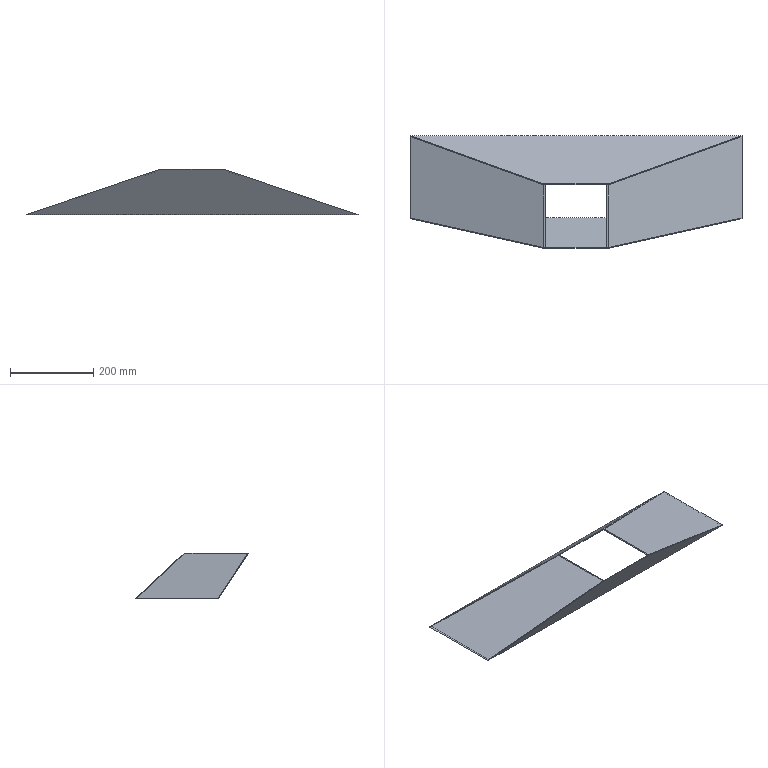Part | SolidWorks | features BaseBody 4 | 4 solids | 26 faces | box 800 x 271.5 x 109 mm | volume 384675 mm3 | plane 26
STEP:
#1=CARTESIAN_POINT('',(-400.,-98.206,0.));
#2=VERTEX_POINT('',#1);
#3=CARTESIAN_POINT('',(400.,-98.206,0.));
#4=VERTEX_POINT('',#3);
#5=CARTESIAN_POINT('',(0.,-98.206,0.));
#6=DIRECTION('',(1.,0.,0.));
#7=VECTOR('',#6,1000.);
#8=LINE('',#5,#7);
#9=EDGE_CURVE('',#2,#4,#8,.T.);
#10=ORIENTED_EDGE('',*,*,#9,.F.);
#11=CARTESIAN_POINT('',(-77.5,-169.706,109.));
#12=VERTEX_POINT('',#11);
#13=CARTESIAN_POINT('',(-74.891,-170.284,109.882));
#14=DIRECTION('',(-0.9271,0.2055,-0.3134));
#15=VECTOR('',#14,1000.);
#16=LINE('',#13,#15);
#17=EDGE_CURVE('',#12,#2,#16,.T.);
#18=ORIENTED_EDGE('',*,*,#17,.F.);
#19=CARTESIAN_POINT('',(77.5,-169.706,109.));
#20=VERTEX_POINT('',#19);
#21=CARTESIAN_POINT('',(0.,-169.706,109.));
#22=DIRECTION('',(1.,0.,0.));
#23=VECTOR('',#22,1000.);
#24=LINE('',#21,#23);
#25=EDGE_CURVE('',#12,#20,#24,.T.);
#26=ORIENTED_EDGE('',*,*,#25,.T.);
#27=CARTESIAN_POINT('',(74.891,-170.284,109.882));
#28=DIRECTION('',(-0.9271,-0.2055,0.3134));
#29=VECTOR('',#28,1000.);
#30=LINE('',#27,#29);
#31=EDGE_CURVE('',#4,#20,#30,.T.);
#32=ORIENTED_EDGE('',*,*,#31,.F.);
#33=EDGE_LOOP('',(#10,#18,#26,#32));
#34=FACE_OUTER_BOUND('',#33,.T.);
#35=CARTESIAN_POINT('',(-72.815,-169.706,109.));
#36=DIRECTION('',(0.,0.8362,0.5485));
#37=DIRECTION('',(1.,0.,0.));
#38=AXIS2_PLACEMENT_3D('',#35,#36,#37);
#39=PLANE('',#38);
#40=ADVANCED_FACE('',(#34),#39,.T.);
#41=ORIENTED_EDGE('',*,*,#25,.F.);
#42=CARTESIAN_POINT('',(-77.5,-171.5,109.));
#43=VERTEX_POINT('',#42);
#44=CARTESIAN_POINT('',(-77.5,-169.706,109.));
#45=CARTESIAN_POINT('',(-77.5,-170.304,109.));
#46=CARTESIAN_POINT('',(-77.5,-170.902,109.));
#47=CARTESIAN_POINT('',(-77.5,-171.5,109.));
#48=B_SPLINE_CURVE_WITH_KNOTS('',3,(#44,#45,#46,#47),.UNSPECIFIED.,.F.,.F.,(4,4),(0.9884,1.),.UNSPECIFIED.);
#49=EDGE_CURVE('',#12,#43,#48,.T.);
#50=ORIENTED_EDGE('',*,*,#49,.T.);
#51=CARTESIAN_POINT('',(77.5,-171.5,109.));
#52=VERTEX_POINT('',#51);
#53=CARTESIAN_POINT('',(-77.5,-171.5,109.));
#54=CARTESIAN_POINT('',(-25.833,-171.5,109.));
#55=CARTESIAN_POINT('',(25.833,-171.5,109.));
#56=CARTESIAN_POINT('',(77.5,-171.5,109.));
#57=B_SPLINE_CURVE_WITH_KNOTS('',3,(#53,#54,#55,#56),.UNSPECIFIED.,.F.,.F.,(4,4),(0.,1.),.UNSPECIFIED.);
#58=EDGE_CURVE('',#43,#52,#57,.T.);
#59=ORIENTED_EDGE('',*,*,#58,.T.);
#60=CARTESIAN_POINT('',(77.5,-171.5,109.));
#61=CARTESIAN_POINT('',(77.5,-170.902,109.));
#62=CARTESIAN_POINT('',(77.5,-170.304,109.));
#63=CARTESIAN_POINT('',(77.5,-169.706,109.));
#64=B_SPLINE_CURVE_WITH_KNOTS('',3,(#60,#61,#62,#63),.UNSPECIFIED.,.F.,.F.,(4,4),(0.,0.01157),.UNSPECIFIED.);
#65=EDGE_CURVE('',#52,#20,#64,.T.);
#66=ORIENTED_EDGE('',*,*,#65,.T.);
#67=EDGE_LOOP('',(#41,#50,#59,#66));
#68=FACE_OUTER_BOUND('',#67,.T.);
#69=CARTESIAN_POINT('',(0.,0.,109.));
#70=DIRECTION('',(0.,0.,-1.));
#71=DIRECTION('',(0.,-1.,0.));
#72=AXIS2_PLACEMENT_3D('',#69,#70,#71);
#73=PLANE('',#72);
#74=ADVANCED_FACE('',(#68),#73,.F.);
#75=CARTESIAN_POINT('',(-400.,-100.,0.));
#76=VERTEX_POINT('',#75);
#77=CARTESIAN_POINT('',(-400.,-98.206,0.));
#78=CARTESIAN_POINT('',(-400.,-98.804,0.));
#79=CARTESIAN_POINT('',(-400.,-99.402,0.));
#80=CARTESIAN_POINT('',(-400.,-100.,0.));
#81=B_SPLINE_CURVE_WITH_KNOTS('',3,(#77,#78,#79,#80),.UNSPECIFIED.,.F.,.F.,(4,4),(0.991,1.),.UNSPECIFIED.);
#82=EDGE_CURVE('',#2,#76,#81,.T.);
#83=ORIENTED_EDGE('',*,*,#82,.F.);
#84=ORIENTED_EDGE('',*,*,#9,.T.);
#85=CARTESIAN_POINT('',(400.,-100.,0.));
#86=VERTEX_POINT('',#85);
#87=CARTESIAN_POINT('',(400.,-100.,0.));
#88=CARTESIAN_POINT('',(400.,-99.402,0.));
#89=CARTESIAN_POINT('',(400.,-98.804,0.));
#90=CARTESIAN_POINT('',(400.,-98.206,0.));
#91=B_SPLINE_CURVE_WITH_KNOTS('',3,(#87,#88,#89,#90),.UNSPECIFIED.,.F.,.F.,(4,4),(0.,0.00897),.UNSPECIFIED.);
#92=EDGE_CURVE('',#86,#4,#91,.T.);
#93=ORIENTED_EDGE('',*,*,#92,.F.);
#94=CARTESIAN_POINT('',(-400.,-100.,0.));
#95=CARTESIAN_POINT('',(-133.333,-100.,0.));
#96=CARTESIAN_POINT('',(133.333,-100.,0.));
#97=CARTESIAN_POINT('',(400.,-100.,0.));
#98=B_SPLINE_CURVE_WITH_KNOTS('',3,(#94,#95,#96,#97),.UNSPECIFIED.,.F.,.F.,(4,4),(0.,1.),.UNSPECIFIED.);
#99=EDGE_CURVE('',#76,#86,#98,.T.);
#100=ORIENTED_EDGE('',*,*,#99,.F.);
#101=EDGE_LOOP('',(#83,#84,#93,#100));
#102=FACE_OUTER_BOUND('',#101,.T.);
#103=CARTESIAN_POINT('',(0.,0.,0.));
#104=DIRECTION('',(0.,0.,-1.));
#105=DIRECTION('',(0.,-1.,0.));
#106=AXIS2_PLACEMENT_3D('',#103,#104,#105);
#107=PLANE('',#106);
#108=ADVANCED_FACE('',(#102),#107,.T.);
#109=ORIENTED_EDGE('',*,*,#49,.F.);
#110=ORIENTED_EDGE('',*,*,#17,.T.);
#111=ORIENTED_EDGE('',*,*,#82,.T.);
#112=CARTESIAN_POINT('',(-77.5,-171.5,109.));
#113=DIRECTION('',(-0.9271,0.2055,-0.3134));
#114=VECTOR('',#113,1000.);
#115=LINE('',#112,#114);
#116=EDGE_CURVE('',#43,#76,#115,.T.);
#117=ORIENTED_EDGE('',*,*,#116,.F.);
#118=EDGE_LOOP('',(#109,#110,#111,#117));
#119=FACE_OUTER_BOUND('',#118,.T.);
#120=CARTESIAN_POINT('',(-41.009,0.,121.333));
#121=DIRECTION('',(-0.3202,0.,0.9474));
#122=DIRECTION('',(0.,1.,0.));
#123=AXIS2_PLACEMENT_3D('',#120,#121,#122);
#124=PLANE('',#123);
#125=ADVANCED_FACE('',(#119),#124,.T.);
#126=ORIENTED_EDGE('',*,*,#92,.T.);
#127=ORIENTED_EDGE('',*,*,#31,.T.);
#128=ORIENTED_EDGE('',*,*,#65,.F.);
#129=CARTESIAN_POINT('',(77.5,-171.5,109.));
#130=DIRECTION('',(0.9271,0.2055,-0.3134));
#131=VECTOR('',#130,1000.);
#132=LINE('',#129,#131);
#133=EDGE_CURVE('',#52,#86,#132,.T.);
#134=ORIENTED_EDGE('',*,*,#133,.T.);
#135=EDGE_LOOP('',(#126,#127,#128,#134));
#136=FACE_OUTER_BOUND('',#135,.T.);
#137=CARTESIAN_POINT('',(41.009,0.,121.333));
#138=DIRECTION('',(0.3202,0.,0.9474));
#139=DIRECTION('',(0.,-1.,0.));
#140=AXIS2_PLACEMENT_3D('',#137,#138,#139);
#141=PLANE('',#140);
#142=ADVANCED_FACE('',(#136),#141,.T.);
#143=ORIENTED_EDGE('',*,*,#116,.T.);
#144=ORIENTED_EDGE('',*,*,#99,.T.);
#145=ORIENTED_EDGE('',*,*,#133,.F.);
#146=ORIENTED_EDGE('',*,*,#58,.F.);
#147=EDGE_LOOP('',(#143,#144,#145,#146));
#148=FACE_OUTER_BOUND('',#147,.T.);
#149=CARTESIAN_POINT('',(0.,-69.916,-45.862));
#150=DIRECTION('',(0.,-0.8362,-0.5485));
#151=DIRECTION('',(0.,0.5485,-0.8362));
#152=AXIS2_PLACEMENT_3D('',#149,#150,#151);
#153=PLANE('',#152);
#154=ADVANCED_FACE('',(#148),#153,.T.);
#155=CLOSED_SHELL('',(#40,#74,#108,#125,#142,#154));
#156=MANIFOLD_SOLID_BREP('',#155);
#157=CARTESIAN_POINT('',(-400.,97.804,0.));
#158=VERTEX_POINT('',#157);
#159=CARTESIAN_POINT('',(-77.5,-18.696,109.));
#160=VERTEX_POINT('',#159);
#161=CARTESIAN_POINT('',(-50.26,-28.536,118.207));
#162=DIRECTION('',(0.8963,-0.3238,0.3029));
#163=VECTOR('',#162,1000.);
#164=LINE('',#161,#163);
#165=EDGE_CURVE('',#158,#160,#164,.T.);
#166=ORIENTED_EDGE('',*,*,#165,.F.);
#167=CARTESIAN_POINT('',(400.,97.804,0.));
#168=VERTEX_POINT('',#167);
#169=CARTESIAN_POINT('',(0.,97.804,0.));
#170=DIRECTION('',(-1.,0.,0.));
#171=VECTOR('',#170,1000.);
#172=LINE('',#169,#171);
#173=EDGE_CURVE('',#168,#158,#172,.T.);
#174=ORIENTED_EDGE('',*,*,#173,.F.);
#175=CARTESIAN_POINT('',(77.5,-18.696,109.));
#176=VERTEX_POINT('',#175);
#177=CARTESIAN_POINT('',(50.26,-28.536,118.207));
#178=DIRECTION('',(0.8963,0.3238,-0.3029));
#179=VECTOR('',#178,1000.);
#180=LINE('',#177,#179);
#181=EDGE_CURVE('',#176,#168,#180,.T.);
#182=ORIENTED_EDGE('',*,*,#181,.F.);
#183=CARTESIAN_POINT('',(0.,-18.696,109.));
#184=DIRECTION('',(-1.,0.,0.));
#185=VECTOR('',#184,1000.);
#186=LINE('',#183,#185);
#187=EDGE_CURVE('',#176,#160,#186,.T.);
#188=ORIENTED_EDGE('',*,*,#187,.T.);
#189=EDGE_LOOP('',(#166,#174,#182,#188));
#190=FACE_OUTER_BOUND('',#189,.T.);
#191=CARTESIAN_POINT('',(72.815,-18.696,109.));
#192=DIRECTION('',(0.,-0.6832,-0.7302));
#193=DIRECTION('',(0.,-0.7302,0.6832));
#194=AXIS2_PLACEMENT_3D('',#191,#192,#193);
#195=PLANE('',#194);
#196=ADVANCED_FACE('',(#190),#195,.T.);
#197=CARTESIAN_POINT('',(77.5,-16.5,109.));
#198=VERTEX_POINT('',#197);
#199=CARTESIAN_POINT('',(400.,100.,0.));
#200=VERTEX_POINT('',#199);
#201=CARTESIAN_POINT('',(77.5,-16.5,109.));
#202=DIRECTION('',(0.8963,0.3238,-0.3029));
#203=VECTOR('',#202,1000.);
#204=LINE('',#201,#203);
#205=EDGE_CURVE('',#198,#200,#204,.T.);
#206=ORIENTED_EDGE('',*,*,#205,.T.);
#207=CARTESIAN_POINT('',(-400.,100.,0.));
#208=VERTEX_POINT('',#207);
#209=CARTESIAN_POINT('',(400.,100.,0.));
#210=CARTESIAN_POINT('',(133.333,100.,0.));
#211=CARTESIAN_POINT('',(-133.333,100.,0.));
#212=CARTESIAN_POINT('',(-400.,100.,0.));
#213=B_SPLINE_CURVE_WITH_KNOTS('',3,(#209,#210,#211,#212),.UNSPECIFIED.,.F.,.F.,(4,4),(0.,1.),.UNSPECIFIED.);
#214=EDGE_CURVE('',#200,#208,#213,.T.);
#215=ORIENTED_EDGE('',*,*,#214,.T.);
#216=CARTESIAN_POINT('',(-77.5,-16.5,109.));
#217=VERTEX_POINT('',#216);
#218=CARTESIAN_POINT('',(-77.5,-16.5,109.));
#219=DIRECTION('',(-0.8963,0.3238,-0.3029));
#220=VECTOR('',#219,1000.);
#221=LINE('',#218,#220);
#222=EDGE_CURVE('',#217,#208,#221,.T.);
#223=ORIENTED_EDGE('',*,*,#222,.F.);
#224=CARTESIAN_POINT('',(77.5,-16.5,109.));
#225=CARTESIAN_POINT('',(25.833,-16.5,109.));
#226=CARTESIAN_POINT('',(-25.833,-16.5,109.));
#227=CARTESIAN_POINT('',(-77.5,-16.5,109.));
#228=B_SPLINE_CURVE_WITH_KNOTS('',3,(#224,#225,#226,#227),.UNSPECIFIED.,.F.,.F.,(4,4),(0.,1.),.UNSPECIFIED.);
#229=EDGE_CURVE('',#198,#217,#228,.T.);
#230=ORIENTED_EDGE('',*,*,#229,.F.);
#231=EDGE_LOOP('',(#206,#215,#223,#230));
#232=FACE_OUTER_BOUND('',#231,.T.);
#233=CARTESIAN_POINT('',(0.,46.678,49.89));
#234=DIRECTION('',(0.,0.6832,0.7302));
#235=DIRECTION('',(1.,0.,0.));
#236=AXIS2_PLACEMENT_3D('',#233,#234,#235);
#237=PLANE('',#236);
#238=ADVANCED_FACE('',(#232),#237,.T.);
#239=CARTESIAN_POINT('',(77.5,-18.696,109.));
#240=CARTESIAN_POINT('',(77.5,-17.964,109.));
#241=CARTESIAN_POINT('',(77.5,-17.232,109.));
#242=CARTESIAN_POINT('',(77.5,-16.5,109.));
#243=B_SPLINE_CURVE_WITH_KNOTS('',3,(#239,#240,#241,#242),.UNSPECIFIED.,.F.,.F.,(4,4),(0.9858,1.),.UNSPECIFIED.);
#244=EDGE_CURVE('',#176,#198,#243,.T.);
#245=ORIENTED_EDGE('',*,*,#244,.F.);
#246=ORIENTED_EDGE('',*,*,#181,.T.);
#247=CARTESIAN_POINT('',(400.,97.804,0.));
#248=CARTESIAN_POINT('',(400.,98.536,0.));
#249=CARTESIAN_POINT('',(400.,99.268,0.));
#250=CARTESIAN_POINT('',(400.,100.,0.));
#251=B_SPLINE_CURVE_WITH_KNOTS('',3,(#247,#248,#249,#250),.UNSPECIFIED.,.F.,.F.,(4,4),(0.989,1.),.UNSPECIFIED.);
#252=EDGE_CURVE('',#168,#200,#251,.T.);
#253=ORIENTED_EDGE('',*,*,#252,.T.);
#254=ORIENTED_EDGE('',*,*,#205,.F.);
#255=EDGE_LOOP('',(#245,#246,#253,#254));
#256=FACE_OUTER_BOUND('',#255,.T.);
#257=CARTESIAN_POINT('',(41.009,0.,121.333));
#258=DIRECTION('',(0.3202,0.,0.9474));
#259=DIRECTION('',(0.,-1.,0.));
#260=AXIS2_PLACEMENT_3D('',#257,#258,#259);
#261=PLANE('',#260);
#262=ADVANCED_FACE('',(#256),#261,.T.);
#263=CARTESIAN_POINT('',(-400.,100.,0.));
#264=CARTESIAN_POINT('',(-400.,99.268,0.));
#265=CARTESIAN_POINT('',(-400.,98.536,0.));
#266=CARTESIAN_POINT('',(-400.,97.804,0.));
#267=B_SPLINE_CURVE_WITH_KNOTS('',3,(#263,#264,#265,#266),.UNSPECIFIED.,.F.,.F.,(4,4),(0.,0.01098),.UNSPECIFIED.);
#268=EDGE_CURVE('',#208,#158,#267,.T.);
#269=ORIENTED_EDGE('',*,*,#268,.T.);
#270=ORIENTED_EDGE('',*,*,#165,.T.);
#271=CARTESIAN_POINT('',(-77.5,-16.5,109.));
#272=CARTESIAN_POINT('',(-77.5,-17.232,109.));
#273=CARTESIAN_POINT('',(-77.5,-17.964,109.));
#274=CARTESIAN_POINT('',(-77.5,-18.696,109.));
#275=B_SPLINE_CURVE_WITH_KNOTS('',3,(#271,#272,#273,#274),.UNSPECIFIED.,.F.,.F.,(4,4),(0.,0.01416),.UNSPECIFIED.);
#276=EDGE_CURVE('',#217,#160,#275,.T.);
#277=ORIENTED_EDGE('',*,*,#276,.F.);
#278=ORIENTED_EDGE('',*,*,#222,.T.);
#279=EDGE_LOOP('',(#269,#270,#277,#278));
#280=FACE_OUTER_BOUND('',#279,.T.);
#281=CARTESIAN_POINT('',(-41.009,0.,121.333));
#282=DIRECTION('',(-0.3202,0.,0.9474));
#283=DIRECTION('',(0.,1.,0.));
#284=AXIS2_PLACEMENT_3D('',#281,#282,#283);
#285=PLANE('',#284);
#286=ADVANCED_FACE('',(#280),#285,.T.);
#287=ORIENTED_EDGE('',*,*,#187,.F.);
#288=ORIENTED_EDGE('',*,*,#244,.T.);
#289=ORIENTED_EDGE('',*,*,#229,.T.);
#290=ORIENTED_EDGE('',*,*,#276,.T.);
#291=EDGE_LOOP('',(#287,#288,#289,#290));
#292=FACE_OUTER_BOUND('',#291,.T.);
#293=CARTESIAN_POINT('',(0.,0.,109.));
#294=DIRECTION('',(0.,0.,-1.));
#295=DIRECTION('',(0.,-1.,0.));
#296=AXIS2_PLACEMENT_3D('',#293,#294,#295);
#297=PLANE('',#296);
#298=ADVANCED_FACE('',(#292),#297,.F.);
#299=ORIENTED_EDGE('',*,*,#252,.F.);
#300=ORIENTED_EDGE('',*,*,#173,.T.);
#301=ORIENTED_EDGE('',*,*,#268,.F.);
#302=ORIENTED_EDGE('',*,*,#214,.F.);
#303=EDGE_LOOP('',(#299,#300,#301,#302));
#304=FACE_OUTER_BOUND('',#303,.T.);
#305=CARTESIAN_POINT('',(0.,0.,0.));
#306=DIRECTION('',(0.,0.,-1.));
#307=DIRECTION('',(0.,-1.,0.));
#308=AXIS2_PLACEMENT_3D('',#305,#306,#307);
#309=PLANE('',#308);
#310=ADVANCED_FACE('',(#304),#309,.T.);
#311=CLOSED_SHELL('',(#196,#238,#262,#286,#298,#310));
#312=MANIFOLD_SOLID_BREP('',#311);
#313=CARTESIAN_POINT('',(74.615,-169.706,109.));
#314=VERTEX_POINT('',#313);
#315=CARTESIAN_POINT('',(74.615,-18.696,109.));
#316=VERTEX_POINT('',#315);
#317=CARTESIAN_POINT('',(74.615,0.,109.));
#318=DIRECTION('',(0.,1.,0.));
#319=VECTOR('',#318,1000.);
#320=LINE('',#317,#319);
#321=EDGE_CURVE('',#314,#316,#320,.T.);
#322=ORIENTED_EDGE('',*,*,#321,.T.);
#323=CARTESIAN_POINT('',(74.615,-18.045,108.392));
#324=VERTEX_POINT('',#323);
#325=CARTESIAN_POINT('',(74.615,-11.983,102.72));
#326=DIRECTION('',(0.,-0.7302,0.6832));
#327=VECTOR('',#326,1000.);
#328=LINE('',#325,#327);
#329=EDGE_CURVE('',#324,#316,#328,.T.);
#330=ORIENTED_EDGE('',*,*,#329,.F.);
#331=CARTESIAN_POINT('',(74.615,-169.307,108.392));
#332=VERTEX_POINT('',#331);
#333=CARTESIAN_POINT('',(74.615,0.,108.392));
#334=DIRECTION('',(0.,-1.,0.));
#335=VECTOR('',#334,1000.);
#336=LINE('',#333,#335);
#337=EDGE_CURVE('',#324,#332,#336,.T.);
#338=ORIENTED_EDGE('',*,*,#337,.T.);
#339=CARTESIAN_POINT('',(74.615,-165.587,102.72));
#340=DIRECTION('',(0.,0.5485,-0.8362));
#341=VECTOR('',#340,1000.);
#342=LINE('',#339,#341);
#343=EDGE_CURVE('',#314,#332,#342,.T.);
#344=ORIENTED_EDGE('',*,*,#343,.F.);
#345=EDGE_LOOP('',(#322,#330,#338,#344));
#346=FACE_OUTER_BOUND('',#345,.T.);
#347=CARTESIAN_POINT('',(74.615,0.,0.));
#348=DIRECTION('',(-1.,0.,0.));
#349=DIRECTION('',(0.,0.,1.));
#350=AXIS2_PLACEMENT_3D('',#347,#348,#349);
#351=PLANE('',#350);
#352=ADVANCED_FACE('',(#346),#351,.T.);
#353=CARTESIAN_POINT('',(400.,97.804,0.));
#354=VERTEX_POINT('',#353);
#355=CARTESIAN_POINT('',(395.315,97.804,0.));
#356=VERTEX_POINT('',#355);
#357=CARTESIAN_POINT('',(0.,97.804,0.));
#358=DIRECTION('',(-1.,0.,0.));
#359=VECTOR('',#358,1000.);
#360=LINE('',#357,#359);
#361=EDGE_CURVE('',#354,#356,#360,.T.);
#362=ORIENTED_EDGE('',*,*,#361,.F.);
#363=CARTESIAN_POINT('',(400.,-98.206,0.));
#364=VERTEX_POINT('',#363);
#365=CARTESIAN_POINT('',(400.,-98.206,0.));
#366=CARTESIAN_POINT('',(400.,-32.869,0.));
#367=CARTESIAN_POINT('',(400.,32.468,0.));
#368=CARTESIAN_POINT('',(400.,97.804,0.));
#369=B_SPLINE_CURVE_WITH_KNOTS('',3,(#365,#366,#367,#368),.UNSPECIFIED.,.F.,.F.,(4,4),(0.00897,0.989),.UNSPECIFIED.);
#370=EDGE_CURVE('',#364,#354,#369,.T.);
#371=ORIENTED_EDGE('',*,*,#370,.F.);
#372=CARTESIAN_POINT('',(395.315,-98.206,0.));
#373=VERTEX_POINT('',#372);
#374=CARTESIAN_POINT('',(0.,-98.206,0.));
#375=DIRECTION('',(1.,0.,0.));
#376=VECTOR('',#375,1000.);
#377=LINE('',#374,#376);
#378=EDGE_CURVE('',#373,#364,#377,.T.);
#379=ORIENTED_EDGE('',*,*,#378,.F.);
#380=CARTESIAN_POINT('',(395.315,0.,0.));
#381=DIRECTION('',(0.,1.,0.));
#382=VECTOR('',#381,1000.);
#383=LINE('',#380,#382);
#384=EDGE_CURVE('',#373,#356,#383,.T.);
#385=ORIENTED_EDGE('',*,*,#384,.T.);
#386=EDGE_LOOP('',(#362,#371,#379,#385));
#387=FACE_OUTER_BOUND('',#386,.T.);
#388=CARTESIAN_POINT('',(0.,0.,0.));
#389=DIRECTION('',(0.,0.,-1.));
#390=DIRECTION('',(0.,-1.,0.));
#391=AXIS2_PLACEMENT_3D('',#388,#389,#390);
#392=PLANE('',#391);
#393=ADVANCED_FACE('',(#387),#392,.T.);
#394=CARTESIAN_POINT('',(77.5,-18.696,109.));
#395=VERTEX_POINT('',#394);
#396=CARTESIAN_POINT('',(50.26,-28.536,118.207));
#397=DIRECTION('',(0.8963,0.3238,-0.3029));
#398=VECTOR('',#397,1000.);
#399=LINE('',#396,#398);
#400=EDGE_CURVE('',#395,#354,#399,.T.);
#401=ORIENTED_EDGE('',*,*,#400,.F.);
#402=CARTESIAN_POINT('',(77.5,-169.706,109.));
#403=VERTEX_POINT('',#402);
#404=CARTESIAN_POINT('',(77.5,-169.706,109.));
#405=CARTESIAN_POINT('',(77.5,-119.369,109.));
#406=CARTESIAN_POINT('',(77.5,-69.032,109.));
#407=CARTESIAN_POINT('',(77.5,-18.696,109.));
#408=B_SPLINE_CURVE_WITH_KNOTS('',3,(#404,#405,#406,#407),.UNSPECIFIED.,.F.,.F.,(4,4),(0.01157,0.9858),.UNSPECIFIED.);
#409=EDGE_CURVE('',#403,#395,#408,.T.);
#410=ORIENTED_EDGE('',*,*,#409,.F.);
#411=CARTESIAN_POINT('',(74.891,-170.284,109.882));
#412=DIRECTION('',(-0.9271,-0.2055,0.3134));
#413=VECTOR('',#412,1000.);
#414=LINE('',#411,#413);
#415=EDGE_CURVE('',#364,#403,#414,.T.);
#416=ORIENTED_EDGE('',*,*,#415,.F.);
#417=ORIENTED_EDGE('',*,*,#370,.T.);
#418=EDGE_LOOP('',(#401,#410,#416,#417));
#419=FACE_OUTER_BOUND('',#418,.T.);
#420=CARTESIAN_POINT('',(41.009,0.,121.333));
#421=DIRECTION('',(0.3202,0.,0.9474));
#422=DIRECTION('',(0.,-1.,0.));
#423=AXIS2_PLACEMENT_3D('',#420,#421,#422);
#424=PLANE('',#423);
#425=ADVANCED_FACE('',(#419),#424,.T.);
#426=ORIENTED_EDGE('',*,*,#337,.F.);
#427=CARTESIAN_POINT('',(49.339,-27.176,116.935));
#428=DIRECTION('',(0.8963,0.3238,-0.3029));
#429=VECTOR('',#428,1000.);
#430=LINE('',#427,#429);
#431=EDGE_CURVE('',#324,#356,#430,.T.);
#432=ORIENTED_EDGE('',*,*,#431,.T.);
#433=ORIENTED_EDGE('',*,*,#384,.F.);
#434=CARTESIAN_POINT('',(74.233,-169.392,108.521));
#435=DIRECTION('',(0.9271,0.2055,-0.3134));
#436=VECTOR('',#435,1000.);
#437=LINE('',#434,#436);
#438=EDGE_CURVE('',#332,#373,#437,.T.);
#439=ORIENTED_EDGE('',*,*,#438,.F.);
#440=EDGE_LOOP('',(#426,#432,#433,#439));
#441=FACE_OUTER_BOUND('',#440,.T.);
#442=CARTESIAN_POINT('',(40.529,0.,119.912));
#443=DIRECTION('',(0.3202,0.,0.9474));
#444=DIRECTION('',(0.,-1.,0.));
#445=AXIS2_PLACEMENT_3D('',#442,#443,#444);
#446=PLANE('',#445);
#447=ADVANCED_FACE('',(#441),#446,.F.);
#448=ORIENTED_EDGE('',*,*,#343,.T.);
#449=ORIENTED_EDGE('',*,*,#438,.T.);
#450=ORIENTED_EDGE('',*,*,#378,.T.);
#451=ORIENTED_EDGE('',*,*,#415,.T.);
#452=CARTESIAN_POINT('',(0.,-169.706,109.));
#453=DIRECTION('',(1.,0.,0.));
#454=VECTOR('',#453,1000.);
#455=LINE('',#452,#454);
#456=EDGE_CURVE('',#314,#403,#455,.T.);
#457=ORIENTED_EDGE('',*,*,#456,.F.);
#458=EDGE_LOOP('',(#448,#449,#450,#451,#457));
#459=FACE_OUTER_BOUND('',#458,.T.);
#460=CARTESIAN_POINT('',(-72.815,-169.706,109.));
#461=DIRECTION('',(0.,0.8362,0.5485));
#462=DIRECTION('',(1.,0.,0.));
#463=AXIS2_PLACEMENT_3D('',#460,#461,#462);
#464=PLANE('',#463);
#465=ADVANCED_FACE('',(#459),#464,.F.);
#466=ORIENTED_EDGE('',*,*,#321,.F.);
#467=ORIENTED_EDGE('',*,*,#456,.T.);
#468=ORIENTED_EDGE('',*,*,#409,.T.);
#469=CARTESIAN_POINT('',(0.,-18.696,109.));
#470=DIRECTION('',(-1.,0.,0.));
#471=VECTOR('',#470,1000.);
#472=LINE('',#469,#471);
#473=EDGE_CURVE('',#395,#316,#472,.T.);
#474=ORIENTED_EDGE('',*,*,#473,.T.);
#475=EDGE_LOOP('',(#466,#467,#468,#474));
#476=FACE_OUTER_BOUND('',#475,.T.);
#477=CARTESIAN_POINT('',(0.,0.,109.));
#478=DIRECTION('',(0.,0.,-1.));
#479=DIRECTION('',(0.,-1.,0.));
#480=AXIS2_PLACEMENT_3D('',#477,#478,#479);
#481=PLANE('',#480);
#482=ADVANCED_FACE('',(#476),#481,.F.);
#483=ORIENTED_EDGE('',*,*,#329,.T.);
#484=ORIENTED_EDGE('',*,*,#473,.F.);
#485=ORIENTED_EDGE('',*,*,#400,.T.);
#486=ORIENTED_EDGE('',*,*,#361,.T.);
#487=ORIENTED_EDGE('',*,*,#431,.F.);
#488=EDGE_LOOP('',(#483,#484,#485,#486,#487));
#489=FACE_OUTER_BOUND('',#488,.T.);
#490=CARTESIAN_POINT('',(72.815,-18.696,109.));
#491=DIRECTION('',(0.,-0.6832,-0.7302));
#492=DIRECTION('',(0.,-0.7302,0.6832));
#493=AXIS2_PLACEMENT_3D('',#490,#491,#492);
#494=PLANE('',#493);
#495=ADVANCED_FACE('',(#489),#494,.F.);
#496=CLOSED_SHELL('',(#352,#393,#425,#447,#465,#482,#495));
#497=MANIFOLD_SOLID_BREP('',#496);
#498=CARTESIAN_POINT('',(-74.615,-169.706,109.));
#499=VERTEX_POINT('',#498);
#500=CARTESIAN_POINT('',(-74.615,-169.307,108.392));
#501=VERTEX_POINT('',#500);
#502=CARTESIAN_POINT('',(-74.615,-187.171,135.625));
#503=DIRECTION('',(0.,0.5485,-0.8362));
#504=VECTOR('',#503,1000.);
#505=LINE('',#502,#504);
#506=EDGE_CURVE('',#499,#501,#505,.T.);
#507=ORIENTED_EDGE('',*,*,#506,.T.);
#508=CARTESIAN_POINT('',(-74.615,-18.045,108.392));
#509=VERTEX_POINT('',#508);
#510=CARTESIAN_POINT('',(-74.615,0.,108.392));
#511=DIRECTION('',(0.,-1.,0.));
#512=VECTOR('',#511,1000.);
#513=LINE('',#510,#512);
#514=EDGE_CURVE('',#509,#501,#513,.T.);
#515=ORIENTED_EDGE('',*,*,#514,.F.);
#516=CARTESIAN_POINT('',(-74.615,-18.696,109.));
#517=VERTEX_POINT('',#516);
#518=CARTESIAN_POINT('',(-74.615,-11.983,102.72));
#519=DIRECTION('',(0.,-0.7302,0.6832));
#520=VECTOR('',#519,1000.);
#521=LINE('',#518,#520);
#522=EDGE_CURVE('',#509,#517,#521,.T.);
#523=ORIENTED_EDGE('',*,*,#522,.T.);
#524=CARTESIAN_POINT('',(-74.615,0.,109.));
#525=DIRECTION('',(0.,1.,0.));
#526=VECTOR('',#525,1000.);
#527=LINE('',#524,#526);
#528=EDGE_CURVE('',#499,#517,#527,.T.);
#529=ORIENTED_EDGE('',*,*,#528,.F.);
#530=EDGE_LOOP('',(#507,#515,#523,#529));
#531=FACE_OUTER_BOUND('',#530,.T.);
#532=CARTESIAN_POINT('',(-74.615,0.,0.));
#533=DIRECTION('',(-1.,0.,0.));
#534=DIRECTION('',(0.,0.,1.));
#535=AXIS2_PLACEMENT_3D('',#532,#533,#534);
#536=PLANE('',#535);
#537=ADVANCED_FACE('',(#531),#536,.F.);
#538=CARTESIAN_POINT('',(-395.315,97.804,0.));
#539=VERTEX_POINT('',#538);
#540=CARTESIAN_POINT('',(-400.,97.804,0.));
#541=VERTEX_POINT('',#540);
#542=CARTESIAN_POINT('',(0.,97.804,0.));
#543=DIRECTION('',(-1.,0.,0.));
#544=VECTOR('',#543,1000.);
#545=LINE('',#542,#544);
#546=EDGE_CURVE('',#539,#541,#545,.T.);
#547=ORIENTED_EDGE('',*,*,#546,.F.);
#548=CARTESIAN_POINT('',(-395.315,-98.206,0.));
#549=VERTEX_POINT('',#548);
#550=CARTESIAN_POINT('',(-395.315,0.,0.));
#551=DIRECTION('',(0.,-1.,0.));
#552=VECTOR('',#551,1000.);
#553=LINE('',#550,#552);
#554=EDGE_CURVE('',#539,#549,#553,.T.);
#555=ORIENTED_EDGE('',*,*,#554,.T.);
#556=CARTESIAN_POINT('',(-400.,-98.206,0.));
#557=VERTEX_POINT('',#556);
#558=CARTESIAN_POINT('',(0.,-98.206,0.));
#559=DIRECTION('',(1.,0.,0.));
#560=VECTOR('',#559,1000.);
#561=LINE('',#558,#560);
#562=EDGE_CURVE('',#557,#549,#561,.T.);
#563=ORIENTED_EDGE('',*,*,#562,.F.);
#564=CARTESIAN_POINT('',(-400.,97.804,0.));
#565=CARTESIAN_POINT('',(-400.,32.468,0.));
#566=CARTESIAN_POINT('',(-400.,-32.869,0.));
#567=CARTESIAN_POINT('',(-400.,-98.206,0.));
#568=B_SPLINE_CURVE_WITH_KNOTS('',3,(#564,#565,#566,#567),.UNSPECIFIED.,.F.,.F.,(4,4),(0.01098,0.991),.UNSPECIFIED.);
#569=EDGE_CURVE('',#541,#557,#568,.T.);
#570=ORIENTED_EDGE('',*,*,#569,.F.);
#571=EDGE_LOOP('',(#547,#555,#563,#570));
#572=FACE_OUTER_BOUND('',#571,.T.);
#573=CARTESIAN_POINT('',(0.,0.,0.));
#574=DIRECTION('',(0.,0.,-1.));
#575=DIRECTION('',(0.,-1.,0.));
#576=AXIS2_PLACEMENT_3D('',#573,#574,#575);
#577=PLANE('',#576);
#578=ADVANCED_FACE('',(#572),#577,.T.);
#579=CARTESIAN_POINT('',(-74.233,-169.392,108.521));
#580=DIRECTION('',(-0.9271,0.2055,-0.3134));
#581=VECTOR('',#580,1000.);
#582=LINE('',#579,#581);
#583=EDGE_CURVE('',#501,#549,#582,.T.);
#584=ORIENTED_EDGE('',*,*,#583,.F.);
#585=ORIENTED_EDGE('',*,*,#506,.F.);
#586=CARTESIAN_POINT('',(-77.5,-169.706,109.));
#587=VERTEX_POINT('',#586);
#588=CARTESIAN_POINT('',(0.,-169.706,109.));
#589=DIRECTION('',(1.,0.,0.));
#590=VECTOR('',#589,1000.);
#591=LINE('',#588,#590);
#592=EDGE_CURVE('',#587,#499,#591,.T.);
#593=ORIENTED_EDGE('',*,*,#592,.F.);
#594=CARTESIAN_POINT('',(-74.891,-170.284,109.882));
#595=DIRECTION('',(-0.9271,0.2055,-0.3134));
#596=VECTOR('',#595,1000.);
#597=LINE('',#594,#596);
#598=EDGE_CURVE('',#587,#557,#597,.T.);
#599=ORIENTED_EDGE('',*,*,#598,.T.);
#600=ORIENTED_EDGE('',*,*,#562,.T.);
#601=EDGE_LOOP('',(#584,#585,#593,#599,#600));
#602=FACE_OUTER_BOUND('',#601,.T.);
#603=CARTESIAN_POINT('',(-72.815,-169.706,109.));
#604=DIRECTION('',(0.,0.8362,0.5485));
#605=DIRECTION('',(1.,0.,0.));
#606=AXIS2_PLACEMENT_3D('',#603,#604,#605);
#607=PLANE('',#606);
#608=ADVANCED_FACE('',(#602),#607,.F.);
#609=ORIENTED_EDGE('',*,*,#592,.T.);
#610=ORIENTED_EDGE('',*,*,#528,.T.);
#611=CARTESIAN_POINT('',(-77.5,-18.696,109.));
#612=VERTEX_POINT('',#611);
#613=CARTESIAN_POINT('',(0.,-18.696,109.));
#614=DIRECTION('',(-1.,0.,0.));
#615=VECTOR('',#614,1000.);
#616=LINE('',#613,#615);
#617=EDGE_CURVE('',#517,#612,#616,.T.);
#618=ORIENTED_EDGE('',*,*,#617,.T.);
#619=CARTESIAN_POINT('',(-77.5,-18.696,109.));
#620=CARTESIAN_POINT('',(-77.5,-69.032,109.));
#621=CARTESIAN_POINT('',(-77.5,-119.369,109.));
#622=CARTESIAN_POINT('',(-77.5,-169.706,109.));
#623=B_SPLINE_CURVE_WITH_KNOTS('',3,(#619,#620,#621,#622),.UNSPECIFIED.,.F.,.F.,(4,4),(0.01416,0.9884),.UNSPECIFIED.);
#624=EDGE_CURVE('',#612,#587,#623,.T.);
#625=ORIENTED_EDGE('',*,*,#624,.T.);
#626=EDGE_LOOP('',(#609,#610,#618,#625));
#627=FACE_OUTER_BOUND('',#626,.T.);
#628=CARTESIAN_POINT('',(0.,0.,109.));
#629=DIRECTION('',(0.,0.,-1.));
#630=DIRECTION('',(0.,-1.,0.));
#631=AXIS2_PLACEMENT_3D('',#628,#629,#630);
#632=PLANE('',#631);
#633=ADVANCED_FACE('',(#627),#632,.F.);
#634=CARTESIAN_POINT('',(-49.339,-27.176,116.935));
#635=DIRECTION('',(-0.8963,0.3238,-0.3029));
#636=VECTOR('',#635,1000.);
#637=LINE('',#634,#636);
#638=EDGE_CURVE('',#509,#539,#637,.T.);
#639=ORIENTED_EDGE('',*,*,#638,.F.);
#640=ORIENTED_EDGE('',*,*,#514,.T.);
#641=ORIENTED_EDGE('',*,*,#583,.T.);
#642=ORIENTED_EDGE('',*,*,#554,.F.);
#643=EDGE_LOOP('',(#639,#640,#641,#642));
#644=FACE_OUTER_BOUND('',#643,.T.);
#645=CARTESIAN_POINT('',(-40.529,0.,119.912));
#646=DIRECTION('',(-0.3202,0.,0.9474));
#647=DIRECTION('',(0.,1.,0.));
#648=AXIS2_PLACEMENT_3D('',#645,#646,#647);
#649=PLANE('',#648);
#650=ADVANCED_FACE('',(#644),#649,.F.);
#651=CARTESIAN_POINT('',(-50.26,-28.536,118.207));
#652=DIRECTION('',(0.8963,-0.3238,0.3029));
#653=VECTOR('',#652,1000.);
#654=LINE('',#651,#653);
#655=EDGE_CURVE('',#541,#612,#654,.T.);
#656=ORIENTED_EDGE('',*,*,#655,.F.);
#657=ORIENTED_EDGE('',*,*,#569,.T.);
#658=ORIENTED_EDGE('',*,*,#598,.F.);
#659=ORIENTED_EDGE('',*,*,#624,.F.);
#660=EDGE_LOOP('',(#656,#657,#658,#659));
#661=FACE_OUTER_BOUND('',#660,.T.);
#662=CARTESIAN_POINT('',(-41.009,0.,121.333));
#663=DIRECTION('',(-0.3202,0.,0.9474));
#664=DIRECTION('',(0.,1.,0.));
#665=AXIS2_PLACEMENT_3D('',#662,#663,#664);
#666=PLANE('',#665);
#667=ADVANCED_FACE('',(#661),#666,.T.);
#668=ORIENTED_EDGE('',*,*,#617,.F.);
#669=ORIENTED_EDGE('',*,*,#522,.F.);
#670=ORIENTED_EDGE('',*,*,#638,.T.);
#671=ORIENTED_EDGE('',*,*,#546,.T.);
#672=ORIENTED_EDGE('',*,*,#655,.T.);
#673=EDGE_LOOP('',(#668,#669,#670,#671,#672));
#674=FACE_OUTER_BOUND('',#673,.T.);
#675=CARTESIAN_POINT('',(72.815,-18.696,109.));
#676=DIRECTION('',(0.,-0.6832,-0.7302));
#677=DIRECTION('',(0.,-0.7302,0.6832));
#678=AXIS2_PLACEMENT_3D('',#675,#676,#677);
#679=PLANE('',#678);
#680=ADVANCED_FACE('',(#674),#679,.F.);
#681=CLOSED_SHELL('',(#537,#578,#608,#633,#650,#667,#680));
#682=MANIFOLD_SOLID_BREP('',#681);
#683=CARTESIAN_POINT('',(0.,0.,0.));
#684=DIRECTION('',(0.,0.,1.));
#685=DIRECTION('',(1.,0.,0.));
#686=AXIS2_PLACEMENT_3D('',#683,#684,#685);
#687=(LENGTH_UNIT()NAMED_UNIT(*)SI_UNIT(.MILLI.,.METRE.));
#688=UNCERTAINTY_MEASURE_WITH_UNIT(LENGTH_MEASURE(0.00001),#687,'','');
#689=(NAMED_UNIT(*)PLANE_ANGLE_UNIT()SI_UNIT($,.RADIAN.));
#690=(NAMED_UNIT(*)SI_UNIT($,.STERADIAN.)SOLID_ANGLE_UNIT());
#691=(GEOMETRIC_REPRESENTATION_CONTEXT(3)GLOBAL_UNCERTAINTY_ASSIGNED_CONTEXT((#688))GLOBAL_UNIT_ASSIGNED_CONTEXT((#687,#689,#690))REPRESENTATION_CONTEXT('',''));
#692=ADVANCED_BREP_SHAPE_REPRESENTATION('',(#156,#312,#497,#682,#686),#691);